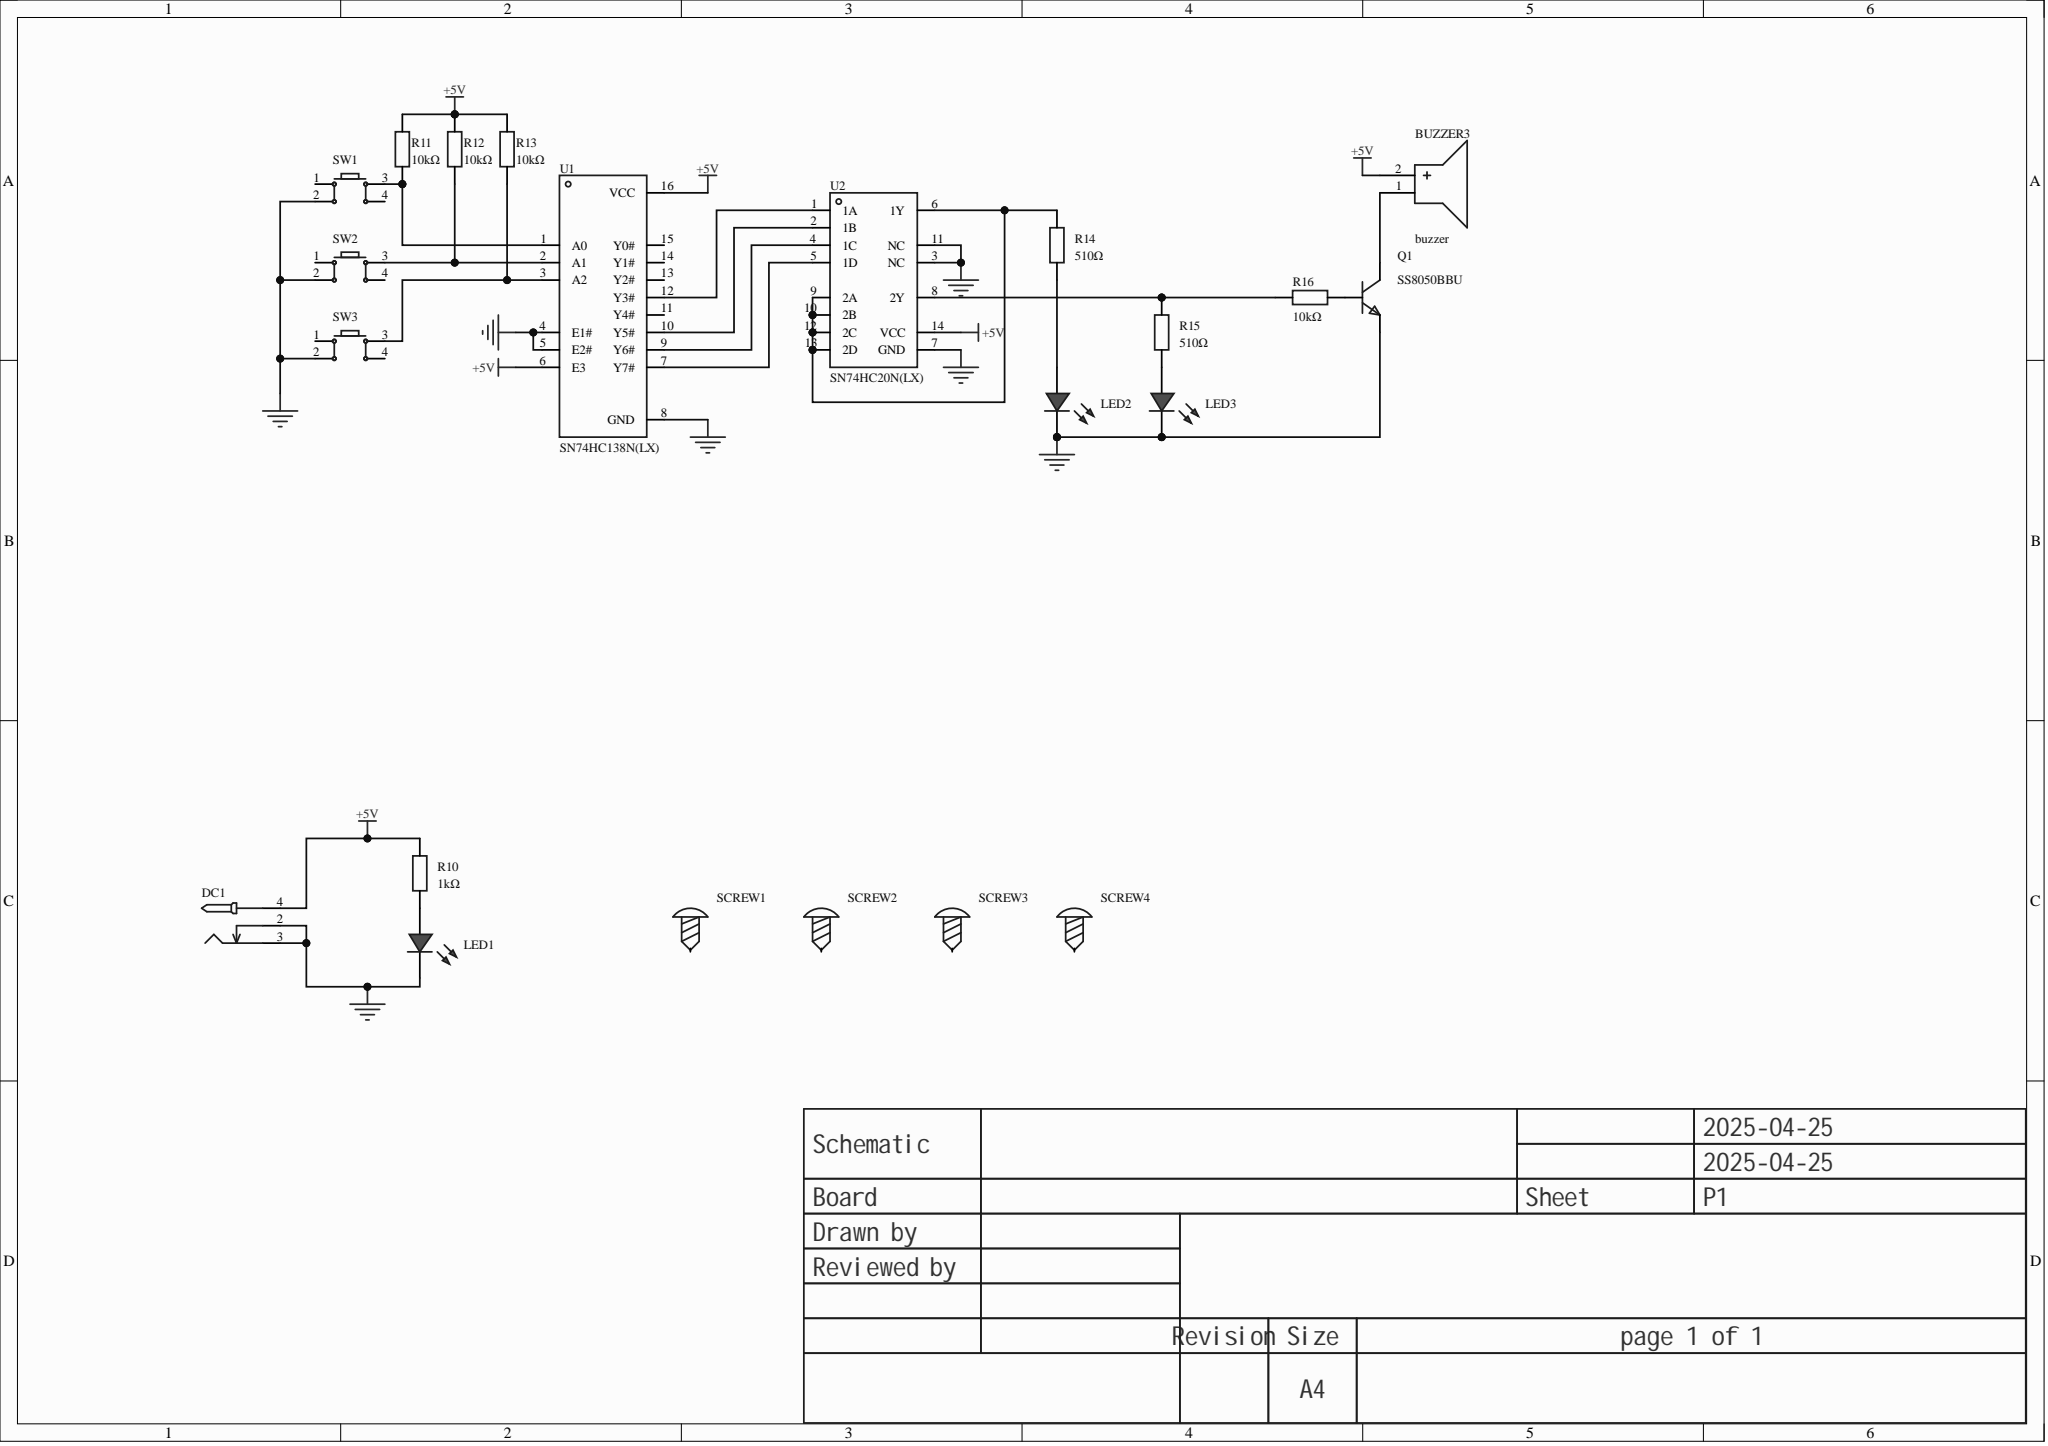Circuit board | Altium Designer | 22 parts | 16 nets
Bill of materials:
Comment,Description,Designator,Footprint,LibRef,Quantity
"buzzer","","BUZZER3","BUZ-TH_BD12.0-P6.00-D0.9-RD","buzzer","1"
"","","DC1","DC-2.0","DC-005_2.0","1"
"","","LED1, LED2, LED3","LED_TH-3mm","LED_TH-R_3mm","3"
"SS8050BBU","","Q1","TO-92-3_L4.8-W3.7-P1.27-L-1","SS8050BBU","1"
"1kΩ","","R10","Res_1/8W","Res_AXIAL-1/8W","1"
"10kΩ","","R11, R12, R13, R16","Res_1/8W","Res_AXIAL-1/8W","4"
"510Ω","","R14, R15","Res_1/8W","Res_AXIAL-1/8W","2"
"","","SCREW1, SCREW2, SCREW3, SCREW4","M3螺丝","M3螺丝","4"
"","","SW1, SW2, SW3","SW-TH_4P-L6.0-W6.0-P4.50-LS6.5","Key_TH_6x6x6","3"
"SN74HC138N(LX)","Operating voltage: 2V~6V;","U1","PDIP-16_L19.3-W6.4-P2.54-LS7.94-BL","SN74HC138N(LX)","1"
"SN74HC20N(LX)","Logic type: NAND gate; channels: 2; operating voltage: 2V~6V; quiescent current (Iq): 2uA; propagation delay (tpd): 15ns@6V,50pF;","U2","PDIP-14_L19.3-W6.5-P2.54-LS7.6-BL","SN74HC20N(LX)","1"
Netlist (Protel format):
[
BUZZER3
BUZ-TH_BD12.0-P6.00-D0.9-RD
buzzer



]
[
DC1
DC-2.0




]
[
LED1
LED_TH-3mm




]
[
LED2
LED_TH-3mm




]
[
LED3
LED_TH-3mm




]
[
Q1
TO-92-3_L4.8-W3.7-P1.27-L-1
SS8050BBU



]
[
R10
Res_1/8W
1kΩ



]
[
R11
Res_1/8W
10kΩ



]
[
R12
Res_1/8W
10kΩ



]
[
R13
Res_1/8W
10kΩ



]
[
R14
Res_1/8W
510Ω



]
[
R15
Res_1/8W
510Ω



]
[
R16
Res_1/8W
10kΩ



]
[
SCREW1
M3螺丝




]
[
SCREW2
M3螺丝




]
[
SCREW3
M3螺丝




]
[
SCREW4
M3螺丝




]
[
SW1
SW-TH_4P-L6.0-W6.0-P4.50-LS6.5




]
[
SW2
SW-TH_4P-L6.0-W6.0-P4.50-LS6.5




]
[
SW3
SW-TH_4P-L6.0-W6.0-P4.50-LS6.5




]
[
U1
PDIP-16_L19.3-W6.4-P2.54-LS7.94-BL
SN74HC138N(LX)



]
[
U2
PDIP-14_L19.3-W6.5-P2.54-LS7.6-BL
SN74HC20N(LX)



]
(
NetU1_12
U1-12
U2-1
)
(
NetU1_10
U1-10
U2-2
)
(
NetU1_9
U1-9
U2-4
)
(
NetU1_7
U1-7
U2-5
)
(
NetR15_2
R15-2
R16-1
U2-8
)
(
NetR14_2
R14-2
U2-6
U2-9
U2-10
U2-12
U2-13
)
(
NetR13_1
R13-1
SW3-3
U1-3
)
(
NetR12_1
R12-1
SW2-3
U1-2
)
(
NetR11_1
R11-1
SW1-3
U1-1
)
(
NetQ1_2
Q1-2
R16-2
)
(
NetLED3_1
LED3-1
R15-1
)
(
NetLED2_1
LED2-1
R14-1
)
(
NetLED1_1
LED1-1
R10-1
)
(
NetBUZZER3_1
BUZZER3-1
Q1-3
)
(
GND
DC1-2
DC1-3
LED1-2
LED2-2
LED3-2
Q1-1
SW1-2
SW2-2
SW3-2
U1-4
U1-5
U1-8
U2-3
U2-7
U2-11
)
(
+5V
BUZZER3-2
DC1-4
R10-2
R11-2
R12-2
R13-2
U1-6
U1-16
U2-14
)